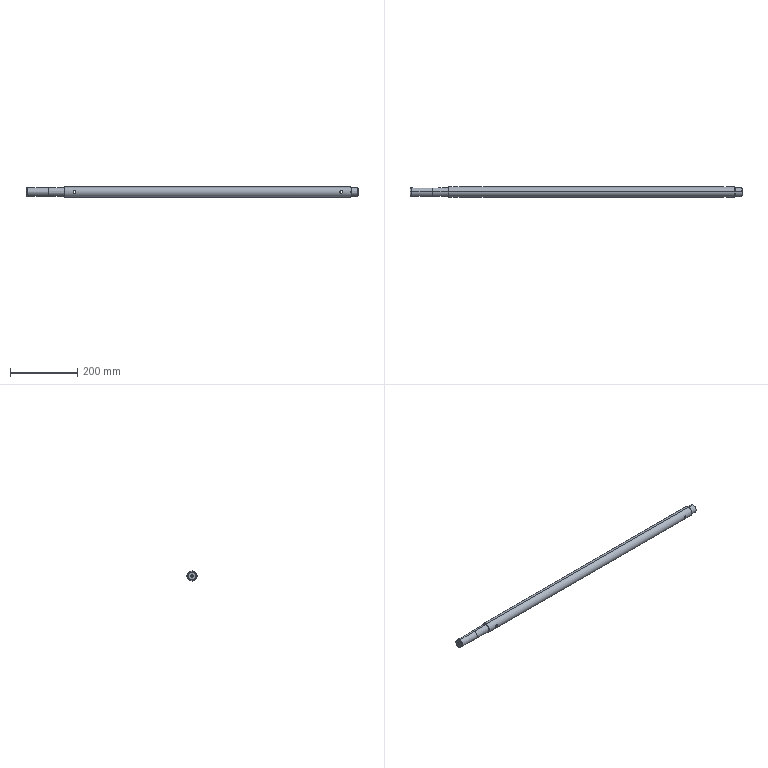Part | SolidWorks | features BaseBody 1 | 1 solid | 42 faces | box 987.5 x 30 x 30 mm | volume 660180 mm3 | cylinder 21 | plane 11 | cone 10 | commonest cylinder face diameters 8 x7 24 x4 25 x4 6.647 x2 22 x2 30 x2